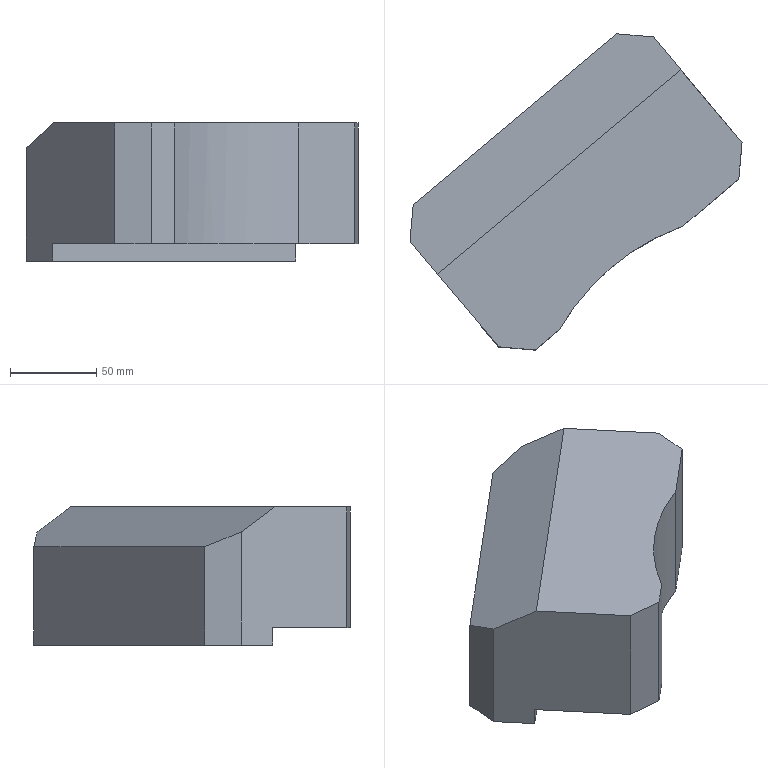Part | NX | features solid 2 | 1 solid | 31 faces | box 192.375 x 183.254 x 80 mm | volume 1312612 mm3 | plane 14 | cylinder 8 | cone 8 | spline 1 | commonest cylinder face diameters 10.579 x4 12 x4
STEP:
#1=CARTESIAN_POINT('',(-593.209,560.45,0.000000024));
#2=VERTEX_POINT('',#1);
#3=CARTESIAN_POINT('',(-598.499,560.45,0.000000024));
#4=DIRECTION('',(0.,0.,1.));
#5=DIRECTION('',(1.,0.,0.));
#6=AXIS2_PLACEMENT_3D('',#3,#4,#5);
#7=CIRCLE('',#6,5.29);
#8=EDGE_CURVE('',#2,#2,#7,.T.);
#9=ORIENTED_EDGE('',*,*,#8,.T.);
#10=EDGE_LOOP('',(#9));
#11=FACE_BOUND('',#10,.T.);
#12=CARTESIAN_POINT('',(-568.696,581.019,0.000000024));
#13=VERTEX_POINT('',#12);
#14=CARTESIAN_POINT('',(-573.985,581.019,0.000000024));
#15=DIRECTION('',(0.,0.,1.));
#16=DIRECTION('',(1.,0.,0.));
#17=AXIS2_PLACEMENT_3D('',#14,#15,#16);
#18=CIRCLE('',#17,5.29);
#19=EDGE_CURVE('',#13,#13,#18,.T.);
#20=ORIENTED_EDGE('',*,*,#19,.T.);
#21=EDGE_LOOP('',(#20));
#22=FACE_BOUND('',#21,.T.);
#23=CARTESIAN_POINT('',(-500.236,592.775,0.000000024));
#24=VERTEX_POINT('',#23);
#25=CARTESIAN_POINT('',(-505.525,592.775,0.000000024));
#26=DIRECTION('',(0.,0.,1.));
#27=DIRECTION('',(1.,0.,0.));
#28=AXIS2_PLACEMENT_3D('',#25,#26,#27);
#29=CIRCLE('',#28,5.29);
#30=EDGE_CURVE('',#24,#24,#29,.T.);
#31=ORIENTED_EDGE('',*,*,#30,.T.);
#32=EDGE_LOOP('',(#31));
#33=FACE_BOUND('',#32,.T.);
#34=CARTESIAN_POINT('',(-616.674,495.071,0.000000024));
#35=VERTEX_POINT('',#34);
#36=CARTESIAN_POINT('',(-621.964,495.071,0.000000024));
#37=DIRECTION('',(0.,0.,1.));
#38=DIRECTION('',(1.,0.,0.));
#39=AXIS2_PLACEMENT_3D('',#36,#37,#38);
#40=CIRCLE('',#39,5.29);
#41=EDGE_CURVE('',#35,#35,#40,.T.);
#42=ORIENTED_EDGE('',*,*,#41,.T.);
#43=EDGE_LOOP('',(#42));
#44=FACE_BOUND('',#43,.T.);
#45=CARTESIAN_POINT('',(-522.023,619.586,0.000000024));
#46=VERTEX_POINT('',#45);
#47=CARTESIAN_POINT('',(-528.023,619.586,0.000000024));
#48=DIRECTION('',(0.,0.,1.));
#49=DIRECTION('',(1.,0.,0.));
#50=AXIS2_PLACEMENT_3D('',#47,#48,#49);
#51=CIRCLE('',#50,6.);
#52=EDGE_CURVE('',#46,#46,#51,.F.);
#53=ORIENTED_EDGE('',*,*,#52,.F.);
#54=EDGE_LOOP('',(#53));
#55=FACE_BOUND('',#54,.T.);
#56=CARTESIAN_POINT('',(-611.65,544.38,0.000000024));
#57=VERTEX_POINT('',#56);
#58=CARTESIAN_POINT('',(-617.65,544.38,0.000000024));
#59=DIRECTION('',(0.,0.,1.));
#60=DIRECTION('',(1.,0.,0.));
#61=AXIS2_PLACEMENT_3D('',#58,#59,#60);
#62=CIRCLE('',#61,6.);
#63=EDGE_CURVE('',#57,#57,#62,.F.);
#64=ORIENTED_EDGE('',*,*,#63,.F.);
#65=EDGE_LOOP('',(#64));
#66=FACE_BOUND('',#65,.T.);
#67=CARTESIAN_POINT('',(-523.703,550.108,0.000000024));
#68=VERTEX_POINT('',#67);
#69=CARTESIAN_POINT('',(-595.572,489.803,0.000000024));
#70=VERTEX_POINT('',#69);
#71=CARTESIAN_POINT('',(-523.703,550.108,0.000000024));
#72=CARTESIAN_POINT('',(-531.205,547.402,0.000000024));
#73=CARTESIAN_POINT('',(-545.792,540.631,0.000000024));
#74=CARTESIAN_POINT('',(-565.448,526.903,0.000000024));
#75=CARTESIAN_POINT('',(-582.431,509.864,0.000000024));
#76=CARTESIAN_POINT('',(-591.599,496.685,0.000000024));
#77=CARTESIAN_POINT('',(-595.572,489.803,0.000000024));
#78=B_SPLINE_CURVE_WITH_KNOTS('',3,(#71,#72,#73,#74,#75,#76,#77),.UNSPECIFIED.,.F.,.F.,(4,1,1,1,4),(0.2128,0.2368,0.2608,0.2847,0.3087),.UNSPECIFIED.);
#79=EDGE_CURVE('',#68,#70,#78,.T.);
#80=ORIENTED_EDGE('',*,*,#79,.T.);
#81=CARTESIAN_POINT('',(-609.231,478.341,0.000000024));
#82=VERTEX_POINT('',#81);
#83=CARTESIAN_POINT('',(-467.513,597.257,0.000000024));
#84=DIRECTION('',(-0.766,-0.6428,0.));
#85=VECTOR('',#84,1000.);
#86=LINE('',#83,#85);
#87=EDGE_CURVE('',#70,#82,#86,.T.);
#88=ORIENTED_EDGE('',*,*,#87,.T.);
#89=CARTESIAN_POINT('',(-630.364,480.19,0.000000024));
#90=VERTEX_POINT('',#89);
#91=CARTESIAN_POINT('',(-630.364,480.19,0.000000024));
#92=DIRECTION('',(0.9962,-0.08716,0.));
#93=VECTOR('',#92,1000.);
#94=LINE('',#91,#93);
#95=EDGE_CURVE('',#82,#90,#94,.F.);
#96=ORIENTED_EDGE('',*,*,#95,.T.);
#97=CARTESIAN_POINT('',(-666.36,523.089,0.000000024));
#98=VERTEX_POINT('',#97);
#99=CARTESIAN_POINT('',(-668.931,526.153,0.000000024));
#100=DIRECTION('',(-0.6428,0.766,0.));
#101=VECTOR('',#100,1000.);
#102=LINE('',#99,#101);
#103=EDGE_CURVE('',#98,#90,#102,.F.);
#104=ORIENTED_EDGE('',*,*,#103,.F.);
#105=CARTESIAN_POINT('',(-525.408,641.362,0.000000024));
#106=VERTEX_POINT('',#105);
#107=CARTESIAN_POINT('',(-513.151,651.646,0.000000024));
#108=DIRECTION('',(0.766,0.6428,0.));
#109=VECTOR('',#108,1000.);
#110=LINE('',#107,#109);
#111=EDGE_CURVE('',#98,#106,#110,.T.);
#112=ORIENTED_EDGE('',*,*,#111,.T.);
#113=CARTESIAN_POINT('',(-489.412,598.463,0.000000024));
#114=VERTEX_POINT('',#113);
#115=CARTESIAN_POINT('',(-527.979,644.426,0.000000024));
#116=DIRECTION('',(-0.6428,0.766,0.));
#117=VECTOR('',#116,1000.);
#118=LINE('',#115,#117);
#119=EDGE_CURVE('',#106,#114,#118,.F.);
#120=ORIENTED_EDGE('',*,*,#119,.T.);
#121=CARTESIAN_POINT('',(-491.261,577.331,0.000000024));
#122=VERTEX_POINT('',#121);
#123=CARTESIAN_POINT('',(-491.261,577.331,0.000000024));
#124=DIRECTION('',(-0.08716,-0.9962,0.));
#125=VECTOR('',#124,1000.);
#126=LINE('',#123,#125);
#127=EDGE_CURVE('',#114,#122,#126,.T.);
#128=ORIENTED_EDGE('',*,*,#127,.T.);
#129=CARTESIAN_POINT('',(-467.513,597.257,0.000000024));
#130=DIRECTION('',(-0.766,-0.6428,0.));
#131=VECTOR('',#130,1000.);
#132=LINE('',#129,#131);
#133=EDGE_CURVE('',#122,#68,#132,.T.);
#134=ORIENTED_EDGE('',*,*,#133,.T.);
#135=EDGE_LOOP('',(#80,#88,#96,#104,#112,#120,#128,#134));
#136=FACE_BOUND('',#135,.T.);
#137=CARTESIAN_POINT('',(-638.461,521.883,0.000000024));
#138=VERTEX_POINT('',#137);
#139=CARTESIAN_POINT('',(-644.461,521.883,0.000000024));
#140=DIRECTION('',(0.,0.,1.));
#141=DIRECTION('',(1.,0.,0.));
#142=AXIS2_PLACEMENT_3D('',#139,#140,#141);
#143=CIRCLE('',#142,6.);
#144=EDGE_CURVE('',#138,#138,#143,.F.);
#145=ORIENTED_EDGE('',*,*,#144,.F.);
#146=EDGE_LOOP('',(#145));
#147=FACE_BOUND('',#146,.T.);
#148=CARTESIAN_POINT('',(-548.834,597.089,0.000000024));
#149=VERTEX_POINT('',#148);
#150=CARTESIAN_POINT('',(-554.834,597.089,0.000000024));
#151=DIRECTION('',(0.,0.,1.));
#152=DIRECTION('',(1.,0.,0.));
#153=AXIS2_PLACEMENT_3D('',#150,#151,#152);
#154=CIRCLE('',#153,6.);
#155=EDGE_CURVE('',#149,#149,#154,.F.);
#156=ORIENTED_EDGE('',*,*,#155,.F.);
#157=EDGE_LOOP('',(#156));
#158=FACE_BOUND('',#157,.T.);
#159=CARTESIAN_POINT('',(-515.722,654.71,0.000000024));
#160=DIRECTION('',(0.,0.,1.));
#161=DIRECTION('',(1.,0.,0.));
#162=AXIS2_PLACEMENT_3D('',#159,#160,#161);
#163=PLANE('',#162);
#164=ADVANCED_FACE('',(#11,#22,#33,#44,#55,#66,#136,#147,#158),#163,.F.);
#165=CARTESIAN_POINT('',(-595.572,489.803,70.));
#166=VERTEX_POINT('',#165);
#167=CARTESIAN_POINT('',(-595.572,489.803,32.5));
#168=DIRECTION('',(0.,0.,1.));
#169=VECTOR('',#168,1000.);
#170=LINE('',#167,#169);
#171=EDGE_CURVE('',#166,#70,#170,.F.);
#172=ORIENTED_EDGE('',*,*,#171,.F.);
#173=CARTESIAN_POINT('',(-609.231,478.341,70.));
#174=VERTEX_POINT('',#173);
#175=CARTESIAN_POINT('',(-583.347,500.061,70.));
#176=DIRECTION('',(0.766,0.6428,0.));
#177=VECTOR('',#176,1000.);
#178=LINE('',#175,#177);
#179=EDGE_CURVE('',#174,#166,#178,.T.);
#180=ORIENTED_EDGE('',*,*,#179,.F.);
#181=CARTESIAN_POINT('',(-609.231,478.341,0.000000024));
#182=DIRECTION('',(0.,0.,-1.));
#183=VECTOR('',#182,1000.);
#184=LINE('',#181,#183);
#185=EDGE_CURVE('',#174,#82,#184,.T.);
#186=ORIENTED_EDGE('',*,*,#185,.T.);
#187=ORIENTED_EDGE('',*,*,#87,.F.);
#188=EDGE_LOOP('',(#172,#180,#186,#187));
#189=FACE_BOUND('',#188,.T.);
#190=CARTESIAN_POINT('',(-467.513,597.257,0.000000024));
#191=DIRECTION('',(-0.6428,0.766,0.));
#192=DIRECTION('',(-0.766,-0.6428,0.));
#193=AXIS2_PLACEMENT_3D('',#190,#191,#192);
#194=PLANE('',#193);
#195=ADVANCED_FACE('',(#189),#194,.F.);
#196=CARTESIAN_POINT('',(-523.703,550.108,70.));
#197=VERTEX_POINT('',#196);
#198=CARTESIAN_POINT('',(-491.261,577.331,70.));
#199=VERTEX_POINT('',#198);
#200=CARTESIAN_POINT('',(-583.347,500.061,70.));
#201=DIRECTION('',(0.766,0.6428,0.));
#202=VECTOR('',#201,1000.);
#203=LINE('',#200,#202);
#204=EDGE_CURVE('',#197,#199,#203,.T.);
#205=ORIENTED_EDGE('',*,*,#204,.F.);
#206=CARTESIAN_POINT('',(-523.703,550.108,0.000000024));
#207=DIRECTION('',(0.,0.,1.));
#208=VECTOR('',#207,1000.);
#209=LINE('',#206,#208);
#210=EDGE_CURVE('',#68,#197,#209,.T.);
#211=ORIENTED_EDGE('',*,*,#210,.F.);
#212=ORIENTED_EDGE('',*,*,#133,.F.);
#213=CARTESIAN_POINT('',(-491.261,577.331,0.000000024));
#214=DIRECTION('',(0.,0.,1.));
#215=VECTOR('',#214,1000.);
#216=LINE('',#213,#215);
#217=EDGE_CURVE('',#122,#199,#216,.T.);
#218=ORIENTED_EDGE('',*,*,#217,.T.);
#219=EDGE_LOOP('',(#205,#211,#212,#218));
#220=FACE_BOUND('',#219,.T.);
#221=CARTESIAN_POINT('',(-467.513,597.257,0.000000024));
#222=DIRECTION('',(-0.6428,0.766,0.));
#223=DIRECTION('',(-0.766,-0.6428,0.));
#224=AXIS2_PLACEMENT_3D('',#221,#222,#223);
#225=PLANE('',#224);
#226=ADVANCED_FACE('',(#220),#225,.F.);
#227=CARTESIAN_POINT('',(-595.572,489.803,70.));
#228=CARTESIAN_POINT('',(-591.553,496.763,70.));
#229=CARTESIAN_POINT('',(-584.704,506.595,70.));
#230=CARTESIAN_POINT('',(-573.845,518.482,70.));
#231=CARTESIAN_POINT('',(-562.131,529.212,70.));
#232=CARTESIAN_POINT('',(-549.111,538.318,70.));
#233=CARTESIAN_POINT('',(-534.819,545.727,70.));
#234=CARTESIAN_POINT('',(-527.454,548.755,70.));
#235=CARTESIAN_POINT('',(-523.703,550.108,70.));
#236=B_SPLINE_CURVE_WITH_KNOTS('',3,(#227,#228,#229,#230,#231,#232,#233,#234,#235),.UNSPECIFIED.,.F.,.F.,(4,1,1,1,1,1,4),(0.02941,0.05349,0.06554,0.07758,0.1017,0.1137,0.1257),.UNSPECIFIED.);
#237=EDGE_CURVE('',#197,#166,#236,.F.);
#238=ORIENTED_EDGE('',*,*,#237,.F.);
#239=ORIENTED_EDGE('',*,*,#204,.T.);
#240=CARTESIAN_POINT('',(-489.412,598.463,70.));
#241=VERTEX_POINT('',#240);
#242=CARTESIAN_POINT('',(-491.261,577.331,70.));
#243=DIRECTION('',(0.08716,0.9962,0.));
#244=VECTOR('',#243,1000.);
#245=LINE('',#242,#244);
#246=EDGE_CURVE('',#199,#241,#245,.T.);
#247=ORIENTED_EDGE('',*,*,#246,.T.);
#248=CARTESIAN_POINT('',(-524.765,640.596,70.));
#249=VERTEX_POINT('',#248);
#250=CARTESIAN_POINT('',(-527.979,644.426,70.));
#251=DIRECTION('',(-0.6428,0.766,0.));
#252=VECTOR('',#251,1000.);
#253=LINE('',#250,#252);
#254=EDGE_CURVE('',#249,#241,#253,.F.);
#255=ORIENTED_EDGE('',*,*,#254,.F.);
#256=CARTESIAN_POINT('',(-665.717,522.323,70.));
#257=VERTEX_POINT('',#256);
#258=CARTESIAN_POINT('',(-654.235,531.957,70.));
#259=DIRECTION('',(0.766,0.6428,0.));
#260=VECTOR('',#259,1000.);
#261=LINE('',#258,#260);
#262=EDGE_CURVE('',#249,#257,#261,.F.);
#263=ORIENTED_EDGE('',*,*,#262,.T.);
#264=CARTESIAN_POINT('',(-630.364,480.19,70.));
#265=VERTEX_POINT('',#264);
#266=CARTESIAN_POINT('',(-662.503,518.492,70.));
#267=DIRECTION('',(-0.6428,0.766,0.));
#268=VECTOR('',#267,1000.);
#269=LINE('',#266,#268);
#270=EDGE_CURVE('',#257,#265,#269,.F.);
#271=ORIENTED_EDGE('',*,*,#270,.T.);
#272=CARTESIAN_POINT('',(-630.364,480.19,70.));
#273=DIRECTION('',(-0.9962,0.08716,0.));
#274=VECTOR('',#273,1000.);
#275=LINE('',#272,#274);
#276=EDGE_CURVE('',#265,#174,#275,.F.);
#277=ORIENTED_EDGE('',*,*,#276,.T.);
#278=ORIENTED_EDGE('',*,*,#179,.T.);
#279=EDGE_LOOP('',(#238,#239,#247,#255,#263,#271,#277,#278));
#280=FACE_BOUND('',#279,.T.);
#281=CARTESIAN_POINT('',(-680.718,563.518,70.));
#282=DIRECTION('',(0.,0.,-1.));
#283=DIRECTION('',(0.08716,0.9962,0.));
#284=AXIS2_PLACEMENT_3D('',#281,#282,#283);
#285=PLANE('',#284);
#286=ADVANCED_FACE('',(#280),#285,.F.);
#287=CARTESIAN_POINT('',(-489.412,598.463,0.000000024));
#288=DIRECTION('',(0.,0.,1.));
#289=VECTOR('',#288,1000.);
#290=LINE('',#287,#289);
#291=EDGE_CURVE('',#241,#114,#290,.F.);
#292=ORIENTED_EDGE('',*,*,#291,.T.);
#293=ORIENTED_EDGE('',*,*,#119,.F.);
#294=CARTESIAN_POINT('',(-525.408,641.362,-10.));
#295=VERTEX_POINT('',#294);
#296=CARTESIAN_POINT('',(-525.408,641.362,0.000000024));
#297=DIRECTION('',(0.,0.,-1.));
#298=VECTOR('',#297,1000.);
#299=LINE('',#296,#298);
#300=EDGE_CURVE('',#295,#106,#299,.F.);
#301=ORIENTED_EDGE('',*,*,#300,.F.);
#302=CARTESIAN_POINT('',(-540.835,659.747,-10.));
#303=VERTEX_POINT('',#302);
#304=CARTESIAN_POINT('',(-550.477,671.237,-10.));
#305=DIRECTION('',(-0.6428,0.766,0.));
#306=VECTOR('',#305,1000.);
#307=LINE('',#304,#306);
#308=EDGE_CURVE('',#303,#295,#307,.F.);
#309=ORIENTED_EDGE('',*,*,#308,.F.);
#310=CARTESIAN_POINT('',(-540.835,659.747,55.566));
#311=VERTEX_POINT('',#310);
#312=CARTESIAN_POINT('',(-540.835,659.747,0.000000024));
#313=DIRECTION('',(0.,0.,-1.));
#314=VECTOR('',#313,1000.);
#315=LINE('',#312,#314);
#316=EDGE_CURVE('',#303,#311,#315,.F.);
#317=ORIENTED_EDGE('',*,*,#316,.T.);
#318=CARTESIAN_POINT('',(-528.609,645.177,66.547));
#319=DIRECTION('',(0.5567,-0.6634,0.5));
#320=VECTOR('',#319,1000.);
#321=LINE('',#318,#320);
#322=EDGE_CURVE('',#311,#249,#321,.T.);
#323=ORIENTED_EDGE('',*,*,#322,.T.);
#324=ORIENTED_EDGE('',*,*,#254,.T.);
#325=EDGE_LOOP('',(#292,#293,#301,#309,#317,#323,#324));
#326=FACE_BOUND('',#325,.T.);
#327=CARTESIAN_POINT('',(-527.979,644.426,0.000000024));
#328=DIRECTION('',(0.766,0.6428,0.));
#329=DIRECTION('',(-0.6428,0.766,0.));
#330=AXIS2_PLACEMENT_3D('',#327,#328,#329);
#331=PLANE('',#330);
#332=ADVANCED_FACE('',(#326),#331,.T.);
#333=CARTESIAN_POINT('',(-681.787,541.474,55.566));
#334=VERTEX_POINT('',#333);
#335=CARTESIAN_POINT('',(-660.996,516.696,74.24));
#336=DIRECTION('',(-0.5567,0.6634,-0.5));
#337=VECTOR('',#336,1000.);
#338=LINE('',#335,#337);
#339=EDGE_CURVE('',#257,#334,#338,.T.);
#340=ORIENTED_EDGE('',*,*,#339,.T.);
#341=CARTESIAN_POINT('',(-681.787,541.474,-10.));
#342=VERTEX_POINT('',#341);
#343=CARTESIAN_POINT('',(-681.787,541.474,-10.));
#344=DIRECTION('',(0.,0.,1.));
#345=VECTOR('',#344,1000.);
#346=LINE('',#343,#345);
#347=EDGE_CURVE('',#334,#342,#346,.F.);
#348=ORIENTED_EDGE('',*,*,#347,.T.);
#349=CARTESIAN_POINT('',(-666.36,523.089,-10.));
#350=VERTEX_POINT('',#349);
#351=CARTESIAN_POINT('',(-691.429,552.964,-10.));
#352=DIRECTION('',(-0.6428,0.766,0.));
#353=VECTOR('',#352,1000.);
#354=LINE('',#351,#353);
#355=EDGE_CURVE('',#342,#350,#354,.F.);
#356=ORIENTED_EDGE('',*,*,#355,.T.);
#357=CARTESIAN_POINT('',(-666.36,523.089,0.000000024));
#358=DIRECTION('',(0.,0.,-1.));
#359=VECTOR('',#358,1000.);
#360=LINE('',#357,#359);
#361=EDGE_CURVE('',#350,#98,#360,.F.);
#362=ORIENTED_EDGE('',*,*,#361,.T.);
#363=ORIENTED_EDGE('',*,*,#103,.T.);
#364=CARTESIAN_POINT('',(-630.364,480.19,60.));
#365=DIRECTION('',(0.,0.,-1.));
#366=VECTOR('',#365,1000.);
#367=LINE('',#364,#366);
#368=EDGE_CURVE('',#90,#265,#367,.F.);
#369=ORIENTED_EDGE('',*,*,#368,.T.);
#370=ORIENTED_EDGE('',*,*,#270,.F.);
#371=EDGE_LOOP('',(#340,#348,#356,#362,#363,#369,#370));
#372=FACE_BOUND('',#371,.T.);
#373=CARTESIAN_POINT('',(-668.931,526.153,0.000000024));
#374=DIRECTION('',(0.766,0.6428,0.));
#375=DIRECTION('',(-0.6428,0.766,0.));
#376=AXIS2_PLACEMENT_3D('',#373,#374,#375);
#377=PLANE('',#376);
#378=ADVANCED_FACE('',(#372),#377,.F.);
#379=CARTESIAN_POINT('',(-679.938,562.606,-10.));
#380=VERTEX_POINT('',#379);
#381=CARTESIAN_POINT('',(-679.938,562.606,46.906));
#382=VERTEX_POINT('',#381);
#383=CARTESIAN_POINT('',(-679.938,562.606,60.));
#384=DIRECTION('',(0.,0.,-1.));
#385=VECTOR('',#384,1000.);
#386=LINE('',#383,#385);
#387=EDGE_CURVE('',#380,#382,#386,.F.);
#388=ORIENTED_EDGE('',*,*,#387,.T.);
#389=CARTESIAN_POINT('',(-561.967,661.596,46.906));
#390=VERTEX_POINT('',#389);
#391=CARTESIAN_POINT('',(-679.946,562.599,46.906));
#392=DIRECTION('',(0.766,0.6428,0.));
#393=VECTOR('',#392,1000.);
#394=LINE('',#391,#393);
#395=EDGE_CURVE('',#382,#390,#394,.T.);
#396=ORIENTED_EDGE('',*,*,#395,.T.);
#397=CARTESIAN_POINT('',(-561.967,661.596,-10.));
#398=VERTEX_POINT('',#397);
#399=CARTESIAN_POINT('',(-561.967,661.596,0.000000024));
#400=DIRECTION('',(0.,0.,1.));
#401=VECTOR('',#400,1000.);
#402=LINE('',#399,#401);
#403=EDGE_CURVE('',#390,#398,#402,.F.);
#404=ORIENTED_EDGE('',*,*,#403,.T.);
#405=CARTESIAN_POINT('',(-668.447,572.248,-10.));
#406=DIRECTION('',(0.766,0.6428,0.));
#407=VECTOR('',#406,1000.);
#408=LINE('',#405,#407);
#409=EDGE_CURVE('',#380,#398,#408,.T.);
#410=ORIENTED_EDGE('',*,*,#409,.F.);
#411=EDGE_LOOP('',(#388,#396,#404,#410));
#412=FACE_BOUND('',#411,.T.);
#413=CARTESIAN_POINT('',(-706.75,540.109,0.000000024));
#414=DIRECTION('',(-0.6428,0.766,0.));
#415=DIRECTION('',(-0.766,-0.6428,0.));
#416=AXIS2_PLACEMENT_3D('',#413,#414,#415);
#417=PLANE('',#416);
#418=ADVANCED_FACE('',(#412),#417,.T.);
#419=ORIENTED_EDGE('',*,*,#409,.T.);
#420=CARTESIAN_POINT('',(-540.835,659.747,-10.));
#421=DIRECTION('',(0.9962,-0.08716,0.));
#422=VECTOR('',#421,1000.);
#423=LINE('',#420,#422);
#424=EDGE_CURVE('',#398,#303,#423,.T.);
#425=ORIENTED_EDGE('',*,*,#424,.T.);
#426=ORIENTED_EDGE('',*,*,#308,.T.);
#427=CARTESIAN_POINT('',(-643.379,542.372,-10.));
#428=DIRECTION('',(-0.766,-0.6428,0.));
#429=VECTOR('',#428,1000.);
#430=LINE('',#427,#429);
#431=EDGE_CURVE('',#350,#295,#430,.F.);
#432=ORIENTED_EDGE('',*,*,#431,.F.);
#433=ORIENTED_EDGE('',*,*,#355,.F.);
#434=CARTESIAN_POINT('',(-679.938,562.606,-10.));
#435=DIRECTION('',(-0.08716,-0.9962,0.));
#436=VECTOR('',#435,1000.);
#437=LINE('',#434,#436);
#438=EDGE_CURVE('',#342,#380,#437,.F.);
#439=ORIENTED_EDGE('',*,*,#438,.T.);
#440=EDGE_LOOP('',(#419,#425,#426,#432,#433,#439));
#441=FACE_BOUND('',#440,.T.);
#442=CARTESIAN_POINT('',(-668.447,572.248,-10.));
#443=DIRECTION('',(0.,0.,-1.));
#444=DIRECTION('',(0.766,0.6428,0.));
#445=AXIS2_PLACEMENT_3D('',#442,#443,#444);
#446=PLANE('',#445);
#447=ADVANCED_FACE('',(#441),#446,.T.);
#448=ORIENTED_EDGE('',*,*,#111,.F.);
#449=ORIENTED_EDGE('',*,*,#361,.F.);
#450=ORIENTED_EDGE('',*,*,#431,.T.);
#451=ORIENTED_EDGE('',*,*,#300,.T.);
#452=EDGE_LOOP('',(#448,#449,#450,#451));
#453=FACE_BOUND('',#452,.T.);
#454=CARTESIAN_POINT('',(-643.379,542.372,-10.));
#455=DIRECTION('',(0.6428,-0.766,0.));
#456=DIRECTION('',(0.766,0.6428,0.));
#457=AXIS2_PLACEMENT_3D('',#454,#455,#456);
#458=PLANE('',#457);
#459=ADVANCED_FACE('',(#453),#458,.T.);
#460=ORIENTED_EDGE('',*,*,#403,.F.);
#461=CARTESIAN_POINT('',(-560.205,661.441,47.628));
#462=DIRECTION('',(0.9223,-0.08069,0.378));
#463=VECTOR('',#462,1000.);
#464=LINE('',#461,#463);
#465=EDGE_CURVE('',#390,#311,#464,.T.);
#466=ORIENTED_EDGE('',*,*,#465,.T.);
#467=ORIENTED_EDGE('',*,*,#316,.F.);
#468=ORIENTED_EDGE('',*,*,#424,.F.);
#469=EDGE_LOOP('',(#460,#466,#467,#468));
#470=FACE_BOUND('',#469,.T.);
#471=CARTESIAN_POINT('',(-540.835,659.747,0.000000024));
#472=DIRECTION('',(-0.08716,-0.9962,0.));
#473=DIRECTION('',(0.9962,-0.08716,0.));
#474=AXIS2_PLACEMENT_3D('',#471,#472,#473);
#475=PLANE('',#474);
#476=ADVANCED_FACE('',(#470),#475,.F.);
#477=ORIENTED_EDGE('',*,*,#347,.F.);
#478=CARTESIAN_POINT('',(-678.508,578.957,40.205));
#479=DIRECTION('',(-0.08069,-0.9223,0.378));
#480=VECTOR('',#479,1000.);
#481=LINE('',#478,#480);
#482=EDGE_CURVE('',#334,#382,#481,.F.);
#483=ORIENTED_EDGE('',*,*,#482,.T.);
#484=ORIENTED_EDGE('',*,*,#387,.F.);
#485=ORIENTED_EDGE('',*,*,#438,.F.);
#486=EDGE_LOOP('',(#477,#483,#484,#485));
#487=FACE_BOUND('',#486,.T.);
#488=CARTESIAN_POINT('',(-679.938,562.606,0.000000024));
#489=DIRECTION('',(-0.9962,0.08716,0.));
#490=DIRECTION('',(-0.08716,-0.9962,0.));
#491=AXIS2_PLACEMENT_3D('',#488,#489,#490);
#492=PLANE('',#491);
#493=ADVANCED_FACE('',(#487),#492,.T.);
#494=ORIENTED_EDGE('',*,*,#95,.F.);
#495=ORIENTED_EDGE('',*,*,#185,.F.);
#496=ORIENTED_EDGE('',*,*,#276,.F.);
#497=ORIENTED_EDGE('',*,*,#368,.F.);
#498=EDGE_LOOP('',(#494,#495,#496,#497));
#499=FACE_BOUND('',#498,.T.);
#500=CARTESIAN_POINT('',(-630.364,480.19,0.000000024));
#501=DIRECTION('',(0.08716,0.9962,0.));
#502=DIRECTION('',(-0.9962,0.08716,0.));
#503=AXIS2_PLACEMENT_3D('',#500,#501,#502);
#504=PLANE('',#503);
#505=ADVANCED_FACE('',(#499),#504,.F.);
#506=ORIENTED_EDGE('',*,*,#127,.F.);
#507=ORIENTED_EDGE('',*,*,#291,.F.);
#508=ORIENTED_EDGE('',*,*,#246,.F.);
#509=ORIENTED_EDGE('',*,*,#217,.F.);
#510=EDGE_LOOP('',(#506,#507,#508,#509));
#511=FACE_BOUND('',#510,.T.);
#512=CARTESIAN_POINT('',(-491.261,577.331,0.000000024));
#513=DIRECTION('',(0.9962,-0.08716,0.));
#514=DIRECTION('',(0.08716,0.9962,0.));
#515=AXIS2_PLACEMENT_3D('',#512,#513,#514);
#516=PLANE('',#515);
#517=ADVANCED_FACE('',(#511),#516,.T.);
#518=ORIENTED_EDGE('',*,*,#465,.F.);
#519=ORIENTED_EDGE('',*,*,#395,.F.);
#520=ORIENTED_EDGE('',*,*,#482,.F.);
#521=ORIENTED_EDGE('',*,*,#339,.F.);
#522=ORIENTED_EDGE('',*,*,#262,.F.);
#523=ORIENTED_EDGE('',*,*,#322,.F.);
#524=EDGE_LOOP('',(#518,#519,#520,#521,#522,#523));
#525=FACE_BOUND('',#524,.T.);
#526=CARTESIAN_POINT('',(-658.079,536.539,66.547));
#527=DIRECTION('',(0.3214,-0.383,-0.866));
#528=DIRECTION('',(-0.8968,0.1706,-0.4082));
#529=AXIS2_PLACEMENT_3D('',#526,#527,#528);
#530=PLANE('',#529);
#531=ADVANCED_FACE('',(#525),#530,.F.);
#532=ORIENTED_EDGE('',*,*,#210,.T.);
#533=ORIENTED_EDGE('',*,*,#237,.T.);
#534=ORIENTED_EDGE('',*,*,#171,.T.);
#535=ORIENTED_EDGE('',*,*,#79,.F.);
#536=EDGE_LOOP('',(#532,#533,#534,#535));
#537=FACE_BOUND('',#536,.T.);
#538=CARTESIAN_POINT('',(-523.703,550.108,0.000000024));
#539=CARTESIAN_POINT('',(-523.703,550.108,70.));
#540=CARTESIAN_POINT('',(-531.233,547.392,0.000000024));
#541=CARTESIAN_POINT('',(-531.233,547.392,70.));
#542=CARTESIAN_POINT('',(-542.036,542.382,0.000000024));
#543=CARTESIAN_POINT('',(-542.036,542.382,70.));
#544=CARTESIAN_POINT('',(-555.597,533.785,0.000000024));
#545=CARTESIAN_POINT('',(-555.597,533.785,70.));
#546=CARTESIAN_POINT('',(-568.47,523.908,0.000000024));
#547=CARTESIAN_POINT('',(-568.47,523.908,70.));
#548=CARTESIAN_POINT('',(-582.535,509.722,0.000000024));
#549=CARTESIAN_POINT('',(-582.535,509.722,70.));
#550=CARTESIAN_POINT('',(-591.647,496.601,0.000000024));
#551=CARTESIAN_POINT('',(-591.647,496.601,70.));
#552=CARTESIAN_POINT('',(-595.572,489.803,0.000000024));
#553=CARTESIAN_POINT('',(-595.572,489.803,70.));
#554=B_SPLINE_SURFACE_WITH_KNOTS('',3,1,((#538,#539),(#540,#541),(#542,#543),(#544,#545),(#546,#547),(#548,#549),(#550,#551),(#552,#553)),.SURF_OF_LINEAR_EXTRUSION.,.F.,.F.,.F.,(4,1,1,1,1,4),(2,2),(0.06717,0.283,0.391,0.4989,0.7148,0.9307),(0.,1.),.UNSPECIFIED.);
#555=ADVANCED_FACE('',(#537),#554,.F.);
#556=ORIENTED_EDGE('',*,*,#144,.T.);
#557=EDGE_LOOP('',(#556));
#558=FACE_BOUND('',#557,.T.);
#559=CARTESIAN_POINT('',(-638.461,521.883,30.));
#560=VERTEX_POINT('',#559);
#561=CARTESIAN_POINT('',(-644.461,521.883,30.));
#562=DIRECTION('',(0.,0.,1.));
#563=DIRECTION('',(1.,0.,0.));
#564=AXIS2_PLACEMENT_3D('',#561,#562,#563);
#565=CIRCLE('',#564,6.);
#566=EDGE_CURVE('',#560,#560,#565,.T.);
#567=ORIENTED_EDGE('',*,*,#566,.T.);
#568=EDGE_LOOP('',(#567));
#569=FACE_BOUND('',#568,.T.);
#570=CARTESIAN_POINT('',(-644.461,521.883,30.));
#571=DIRECTION('',(0.,0.,-1.));
#572=DIRECTION('',(-1.,0.,0.));
#573=AXIS2_PLACEMENT_3D('',#570,#571,#572);
#574=CYLINDRICAL_SURFACE('',#573,6.);
#575=ADVANCED_FACE('',(#558,#569),#574,.F.);
#576=ORIENTED_EDGE('',*,*,#63,.T.);
#577=EDGE_LOOP('',(#576));
#578=FACE_BOUND('',#577,.T.);
#579=CARTESIAN_POINT('',(-611.65,544.38,30.));
#580=VERTEX_POINT('',#579);
#581=CARTESIAN_POINT('',(-617.65,544.38,30.));
#582=DIRECTION('',(0.,0.,1.));
#583=DIRECTION('',(1.,0.,0.));
#584=AXIS2_PLACEMENT_3D('',#581,#582,#583);
#585=CIRCLE('',#584,6.);
#586=EDGE_CURVE('',#580,#580,#585,.T.);
#587=ORIENTED_EDGE('',*,*,#586,.T.);
#588=EDGE_LOOP('',(#587));
#589=FACE_BOUND('',#588,.T.);
#590=CARTESIAN_POINT('',(-617.65,544.38,30.));
#591=DIRECTION('',(0.,0.,-1.));
#592=DIRECTION('',(-1.,0.,0.));
#593=AXIS2_PLACEMENT_3D('',#590,#591,#592);
#594=CYLINDRICAL_SURFACE('',#593,6.);
#595=ADVANCED_FACE('',(#578,#589),#594,.F.);
#596=ORIENTED_EDGE('',*,*,#155,.T.);
#597=EDGE_LOOP('',(#596));
#598=FACE_BOUND('',#597,.T.);
#599=CARTESIAN_POINT('',(-548.834,597.089,30.));
#600=VERTEX_POINT('',#599);
#601=CARTESIAN_POINT('',(-554.834,597.089,30.));
#602=DIRECTION('',(0.,0.,1.));
#603=DIRECTION('',(1.,0.,0.));
#604=AXIS2_PLACEMENT_3D('',#601,#602,#603);
#605=CIRCLE('',#604,6.);
#606=EDGE_CURVE('',#600,#600,#605,.T.);
#607=ORIENTED_EDGE('',*,*,#606,.T.);
#608=EDGE_LOOP('',(#607));
#609=FACE_BOUND('',#608,.T.);
#610=CARTESIAN_POINT('',(-554.834,597.089,30.));
#611=DIRECTION('',(0.,0.,-1.));
#612=DIRECTION('',(-1.,0.,0.));
#613=AXIS2_PLACEMENT_3D('',#610,#611,#612);
#614=CYLINDRICAL_SURFACE('',#613,6.);
#615=ADVANCED_FACE('',(#598,#609),#614,.F.);
#616=ORIENTED_EDGE('',*,*,#52,.T.);
#617=EDGE_LOOP('',(#616));
#618=FACE_BOUND('',#617,.T.);
#619=CARTESIAN_POINT('',(-522.023,619.586,30.));
#620=VERTEX_POINT('',#619);
#621=CARTESIAN_POINT('',(-528.023,619.586,30.));
#622=DIRECTION('',(0.,0.,1.));
#623=DIRECTION('',(1.,0.,0.));
#624=AXIS2_PLACEMENT_3D('',#621,#622,#623);
#625=CIRCLE('',#624,6.);
#626=EDGE_CURVE('',#620,#620,#625,.T.);
#627=ORIENTED_EDGE('',*,*,#626,.T.);
#628=EDGE_LOOP('',(#627));
#629=FACE_BOUND('',#628,.T.);
#630=CARTESIAN_POINT('',(-528.023,619.586,30.));
#631=DIRECTION('',(0.,0.,-1.));
#632=DIRECTION('',(-1.,0.,0.));
#633=AXIS2_PLACEMENT_3D('',#630,#631,#632);
#634=CYLINDRICAL_SURFACE('',#633,6.);
#635=ADVANCED_FACE('',(#618,#629),#634,.F.);
#636=CARTESIAN_POINT('',(-616.674,495.071,30.));
#637=VERTEX_POINT('',#636);
#638=CARTESIAN_POINT('',(-621.964,495.071,30.));
#639=DIRECTION('',(0.,0.,1.));
#640=DIRECTION('',(1.,0.,0.));
#641=AXIS2_PLACEMENT_3D('',#638,#639,#640);
#642=CIRCLE('',#641,5.29);
#643=EDGE_CURVE('',#637,#637,#642,.T.);
#644=ORIENTED_EDGE('',*,*,#643,.F.);
#645=EDGE_LOOP('',(#644));
#646=FACE_BOUND('',#645,.T.);
#647=CARTESIAN_POINT('',(-621.964,495.071,33.178));
#648=VERTEX_POINT('',#647);
#649=VERTEX_LOOP('',#648);
#650=FACE_BOUND('',#649,.T.);
#651=CARTESIAN_POINT('',(-621.964,495.071,30.));
#652=DIRECTION('',(0.,0.,-1.));
#653=DIRECTION('',(-1.,0.,0.));
#654=AXIS2_PLACEMENT_3D('',#651,#652,#653);
#655=CONICAL_SURFACE('',#654,5.29,1.03);
#656=ADVANCED_FACE('',(#646,#650),#655,.F.);
#657=ORIENTED_EDGE('',*,*,#643,.T.);
#658=EDGE_LOOP('',(#657));
#659=FACE_BOUND('',#658,.T.);
#660=ORIENTED_EDGE('',*,*,#41,.F.);
#661=EDGE_LOOP('',(#660));
#662=FACE_BOUND('',#661,.T.);
#663=CARTESIAN_POINT('',(-621.964,495.071,0.000000024));
#664=DIRECTION('',(0.,0.,1.));
#665=DIRECTION('',(1.,0.,0.));
#666=AXIS2_PLACEMENT_3D('',#663,#664,#665);
#667=CYLINDRICAL_SURFACE('',#666,5.29);
#668=ADVANCED_FACE('',(#659,#662),#667,.F.);
#669=CARTESIAN_POINT('',(-500.236,592.775,30.));
#670=VERTEX_POINT('',#669);
#671=CARTESIAN_POINT('',(-505.525,592.775,30.));
#672=DIRECTION('',(0.,0.,1.));
#673=DIRECTION('',(1.,0.,0.));
#674=AXIS2_PLACEMENT_3D('',#671,#672,#673);
#675=CIRCLE('',#674,5.29);
#676=EDGE_CURVE('',#670,#670,#675,.T.);
#677=ORIENTED_EDGE('',*,*,#676,.F.);
#678=EDGE_LOOP('',(#677));
#679=FACE_BOUND('',#678,.T.);
#680=CARTESIAN_POINT('',(-505.525,592.775,33.178));
#681=VERTEX_POINT('',#680);
#682=VERTEX_LOOP('',#681);
#683=FACE_BOUND('',#682,.T.);
#684=CARTESIAN_POINT('',(-505.525,592.775,30.));
#685=DIRECTION('',(0.,0.,-1.));
#686=DIRECTION('',(-1.,0.,0.));
#687=AXIS2_PLACEMENT_3D('',#684,#685,#686);
#688=CONICAL_SURFACE('',#687,5.29,1.03);
#689=ADVANCED_FACE('',(#679,#683),#688,.F.);
#690=ORIENTED_EDGE('',*,*,#676,.T.);
#691=EDGE_LOOP('',(#690));
#692=FACE_BOUND('',#691,.T.);
#693=ORIENTED_EDGE('',*,*,#30,.F.);
#694=EDGE_LOOP('',(#693));
#695=FACE_BOUND('',#694,.T.);
#696=CARTESIAN_POINT('',(-505.525,592.775,0.000000024));
#697=DIRECTION('',(0.,0.,1.));
#698=DIRECTION('',(1.,0.,0.));
#699=AXIS2_PLACEMENT_3D('',#696,#697,#698);
#700=CYLINDRICAL_SURFACE('',#699,5.29);
#701=ADVANCED_FACE('',(#692,#695),#700,.F.);
#702=CARTESIAN_POINT('',(-568.696,581.019,30.));
#703=VERTEX_POINT('',#702);
#704=CARTESIAN_POINT('',(-573.985,581.019,30.));
#705=DIRECTION('',(0.,0.,1.));
#706=DIRECTION('',(1.,0.,0.));
#707=AXIS2_PLACEMENT_3D('',#704,#705,#706);
#708=CIRCLE('',#707,5.29);
#709=EDGE_CURVE('',#703,#703,#708,.T.);
#710=ORIENTED_EDGE('',*,*,#709,.F.);
#711=EDGE_LOOP('',(#710));
#712=FACE_BOUND('',#711,.T.);
#713=CARTESIAN_POINT('',(-573.985,581.019,33.178));
#714=VERTEX_POINT('',#713);
#715=VERTEX_LOOP('',#714);
#716=FACE_BOUND('',#715,.T.);
#717=CARTESIAN_POINT('',(-573.985,581.019,30.));
#718=DIRECTION('',(0.,0.,-1.));
#719=DIRECTION('',(-1.,0.,0.));
#720=AXIS2_PLACEMENT_3D('',#717,#718,#719);
#721=CONICAL_SURFACE('',#720,5.29,1.03);
#722=ADVANCED_FACE('',(#712,#716),#721,.F.);
#723=ORIENTED_EDGE('',*,*,#709,.T.);
#724=EDGE_LOOP('',(#723));
#725=FACE_BOUND('',#724,.T.);
#726=ORIENTED_EDGE('',*,*,#19,.F.);
#727=EDGE_LOOP('',(#726));
#728=FACE_BOUND('',#727,.T.);
#729=CARTESIAN_POINT('',(-573.985,581.019,0.000000024));
#730=DIRECTION('',(0.,0.,1.));
#731=DIRECTION('',(1.,0.,0.));
#732=AXIS2_PLACEMENT_3D('',#729,#730,#731);
#733=CYLINDRICAL_SURFACE('',#732,5.29);
#734=ADVANCED_FACE('',(#725,#728),#733,.F.);
#735=CARTESIAN_POINT('',(-593.209,560.45,30.));
#736=VERTEX_POINT('',#735);
#737=CARTESIAN_POINT('',(-598.499,560.45,30.));
#738=DIRECTION('',(0.,0.,1.));
#739=DIRECTION('',(1.,0.,0.));
#740=AXIS2_PLACEMENT_3D('',#737,#738,#739);
#741=CIRCLE('',#740,5.29);
#742=EDGE_CURVE('',#736,#736,#741,.T.);
#743=ORIENTED_EDGE('',*,*,#742,.F.);
#744=EDGE_LOOP('',(#743));
#745=FACE_BOUND('',#744,.T.);
#746=CARTESIAN_POINT('',(-598.499,560.45,33.178));
#747=VERTEX_POINT('',#746);
#748=VERTEX_LOOP('',#747);
#749=FACE_BOUND('',#748,.T.);
#750=CARTESIAN_POINT('',(-598.499,560.45,30.));
#751=DIRECTION('',(0.,0.,-1.));
#752=DIRECTION('',(-1.,0.,0.));
#753=AXIS2_PLACEMENT_3D('',#750,#751,#752);
#754=CONICAL_SURFACE('',#753,5.29,1.03);
#755=ADVANCED_FACE('',(#745,#749),#754,.F.);
#756=ORIENTED_EDGE('',*,*,#742,.T.);
#757=EDGE_LOOP('',(#756));
#758=FACE_BOUND('',#757,.T.);
#759=ORIENTED_EDGE('',*,*,#8,.F.);
#760=EDGE_LOOP('',(#759));
#761=FACE_BOUND('',#760,.T.);
#762=CARTESIAN_POINT('',(-598.499,560.45,0.000000024));
#763=DIRECTION('',(0.,0.,1.));
#764=DIRECTION('',(1.,0.,0.));
#765=AXIS2_PLACEMENT_3D('',#762,#763,#764);
#766=CYLINDRICAL_SURFACE('',#765,5.29);
#767=ADVANCED_FACE('',(#758,#761),#766,.F.);
#768=ORIENTED_EDGE('',*,*,#586,.F.);
#769=EDGE_LOOP('',(#768));
#770=FACE_BOUND('',#769,.T.);
#771=CARTESIAN_POINT('',(-617.65,544.38,33.605));
#772=VERTEX_POINT('',#771);
#773=VERTEX_LOOP('',#772);
#774=FACE_BOUND('',#773,.T.);
#775=CARTESIAN_POINT('',(-617.65,544.38,30.));
#776=DIRECTION('',(0.,0.,-1.));
#777=DIRECTION('',(-1.,0.,0.));
#778=AXIS2_PLACEMENT_3D('',#775,#776,#777);
#779=CONICAL_SURFACE('',#778,6.,1.03);
#780=ADVANCED_FACE('',(#770,#774),#779,.F.);
#781=ORIENTED_EDGE('',*,*,#566,.F.);
#782=EDGE_LOOP('',(#781));
#783=FACE_BOUND('',#782,.T.);
#784=CARTESIAN_POINT('',(-644.461,521.883,33.605));
#785=VERTEX_POINT('',#784);
#786=VERTEX_LOOP('',#785);
#787=FACE_BOUND('',#786,.T.);
#788=CARTESIAN_POINT('',(-644.461,521.883,30.));
#789=DIRECTION('',(0.,0.,-1.));
#790=DIRECTION('',(-1.,0.,0.));
#791=AXIS2_PLACEMENT_3D('',#788,#789,#790);
#792=CONICAL_SURFACE('',#791,6.,1.03);
#793=ADVANCED_FACE('',(#783,#787),#792,.F.);
#794=ORIENTED_EDGE('',*,*,#606,.F.);
#795=EDGE_LOOP('',(#794));
#796=FACE_BOUND('',#795,.T.);
#797=CARTESIAN_POINT('',(-554.834,597.089,33.605));
#798=VERTEX_POINT('',#797);
#799=VERTEX_LOOP('',#798);
#800=FACE_BOUND('',#799,.T.);
#801=CARTESIAN_POINT('',(-554.834,597.089,30.));
#802=DIRECTION('',(0.,0.,-1.));
#803=DIRECTION('',(-1.,0.,0.));
#804=AXIS2_PLACEMENT_3D('',#801,#802,#803);
#805=CONICAL_SURFACE('',#804,6.,1.03);
#806=ADVANCED_FACE('',(#796,#800),#805,.F.);
#807=ORIENTED_EDGE('',*,*,#626,.F.);
#808=EDGE_LOOP('',(#807));
#809=FACE_BOUND('',#808,.T.);
#810=CARTESIAN_POINT('',(-528.023,619.586,33.605));
#811=VERTEX_POINT('',#810);
#812=VERTEX_LOOP('',#811);
#813=FACE_BOUND('',#812,.T.);
#814=CARTESIAN_POINT('',(-528.023,619.586,30.));
#815=DIRECTION('',(0.,0.,-1.));
#816=DIRECTION('',(-1.,0.,0.));
#817=AXIS2_PLACEMENT_3D('',#814,#815,#816);
#818=CONICAL_SURFACE('',#817,6.,1.03);
#819=ADVANCED_FACE('',(#809,#813),#818,.F.);
#820=CLOSED_SHELL('',(#164,#195,#226,#286,#332,#378,#418,#447,#459,#476,#493,#505,#517,#531,#555,#575,#595,#615,#635,#656,#668,#689,#701,#722,#734,#755,#767,#780,#793,#806,#819));
#821=MANIFOLD_SOLID_BREP('',#820);
#822=(LENGTH_UNIT()NAMED_UNIT(*)SI_UNIT(.MILLI.,.METRE.));
#823=UNCERTAINTY_MEASURE_WITH_UNIT(LENGTH_MEASURE(0.0508),#822,'','');
#824=(NAMED_UNIT(*)PLANE_ANGLE_UNIT()SI_UNIT($,.RADIAN.));
#825=(NAMED_UNIT(*)SI_UNIT($,.STERADIAN.)SOLID_ANGLE_UNIT());
#826=(GEOMETRIC_REPRESENTATION_CONTEXT(3)GLOBAL_UNCERTAINTY_ASSIGNED_CONTEXT((#823))GLOBAL_UNIT_ASSIGNED_CONTEXT((#822,#824,#825))REPRESENTATION_CONTEXT('',''));
#827=ADVANCED_BREP_SHAPE_REPRESENTATION('',(#821),#826);